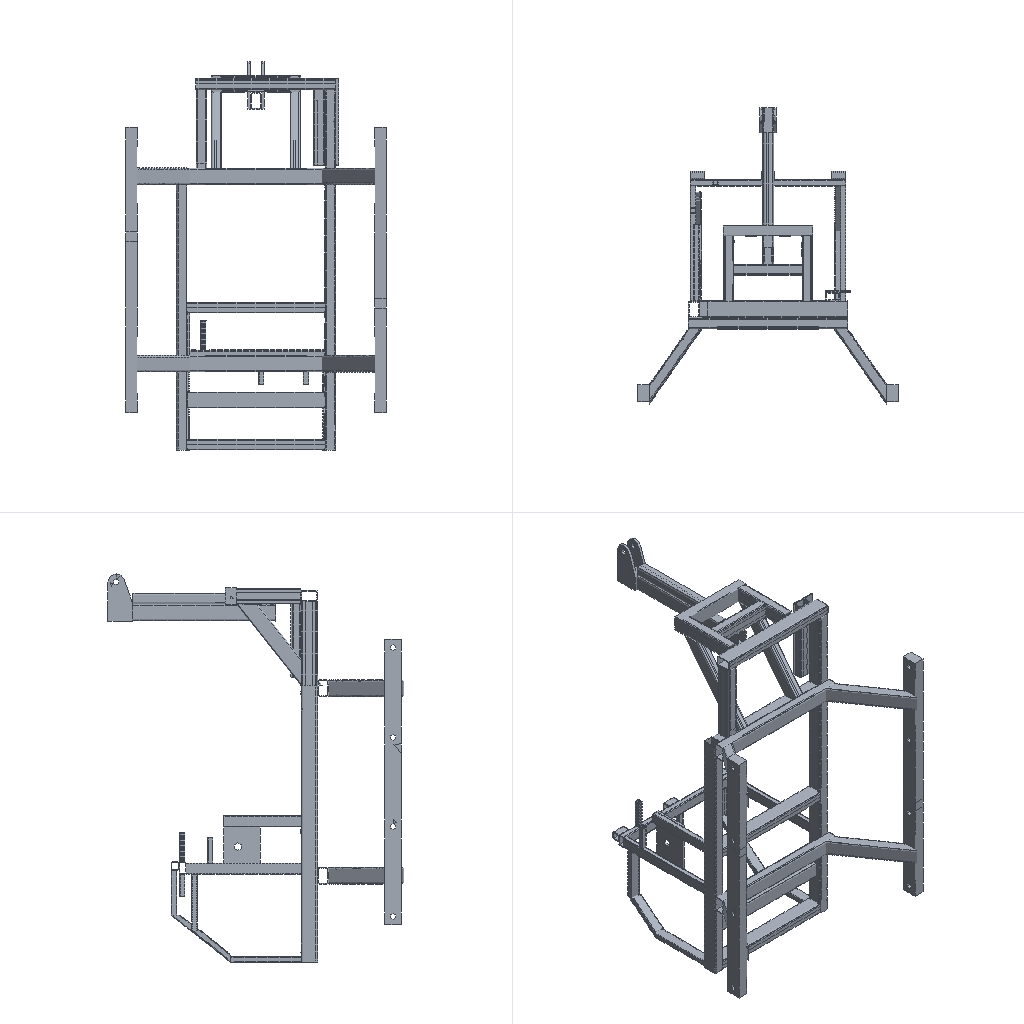Simulation study | ansys workbench
Set-up summary:
category,name,step,type,value,unit,region
solver,ansys_workbench
units,mm-N-s-tonne (MPa),,stated,"/units,MPA"
analysis,LS1,,modal,method=lanb; n_modes=12
load_step,LS1,LS1,modal
mesh,nodes,,,135459
mesh,elements,,,60243
element_type,SOLID187,,,42307
element_type,SOLID186,,,7352
element_type,TARGE170,,,5292
element_type,CONTA174,,,5292
material,Structural Steel,,E,200000,tonne s^-2 mm^-1
material,Structural Steel,,nu,0.3
material,Structural Steel,,density,7.85e-09,tonne mm^-3
material,Structural Steel,,conductivity,60.5,tonne mm s^-3 C^-1
material,Structural Steel,,specific_heat,4.34e+08,mm^2 s^-2 C^-1
material,Structural Steel,,cte,1.2e-05,C^-1
material,Structural Steel,,permeability,10000
material,Structural Steel,,resistivity,0.00017,ohm mm
bc,Fixed Supports,model,fixed,[dofs=ALL],,_FIXEDSU
contact,Contact Region,,bonded (always),element=CONTA174
contact,Contact Region 2,,bonded (always),element=CONTA174
contact,Contact Region 3,,bonded (always),element=CONTA174
contact,Contact Region 4,,bonded (always),element=CONTA174
contact,Contact Region 5,,bonded (always),element=CONTA174
contact,Contact Region 6,,bonded (always),element=CONTA174
contact,Contact Region 7,,bonded (always),element=CONTA174
contact,Contact Region 8,,bonded (always),element=CONTA174
contact,Contact Region 9,,bonded (always),element=CONTA174
contact,Contact Region 10,,bonded (always),element=CONTA174
contact,Contact Region 11,,bonded (always),element=CONTA174
contact,Contact Region 12,,bonded (always),element=CONTA174
contact,Contact Region 13,,bonded (always),element=CONTA174
contact,Contact Region 14,,bonded (always),element=CONTA174
contact,Contact Region 15,,bonded (always),element=CONTA174
contact,Contact Region 16,,bonded (always),element=CONTA174
contact,Contact Region 17,,bonded (always),element=CONTA174
contact,Contact Region 18,,bonded (always),element=CONTA174
contact,Contact Region 19,,bonded (always),element=CONTA174
contact,Contact Region 20,,bonded (always),element=CONTA174
contact,Contact Region 21,,bonded (always),element=CONTA174
contact,Contact Region 22,,bonded (always),element=CONTA174
contact,Contact Region 23,,bonded (always),element=CONTA174
contact,Contact Region 24,,bonded (always),element=CONTA174
contact,Contact Region 25,,bonded (always),element=CONTA174
contact,Contact Region 26,,bonded (always),element=CONTA174
contact,Contact Region 27,,bonded (always),element=CONTA174
contact,Contact Region 28,,bonded (always),element=CONTA174
contact,Contact Region 29,,bonded (always),element=CONTA174
contact,Contact Region 30,,bonded (always),element=CONTA174
contact,Contact Region 31,,bonded (always),element=CONTA174
contact,Contact Region 32,,bonded (always),element=CONTA174
contact,Contact Region 33,,bonded (always),element=CONTA174
contact,Contact Region 34,,bonded (always),element=CONTA174
contact,Contact Region 35,,bonded (always),element=CONTA174
contact,Contact Region 36,,bonded (always),element=CONTA174
contact,Contact Region 37,,bonded (always),element=CONTA174
contact,Contact Region 38,,bonded (always),element=CONTA174
contact,Contact Region 39,,bonded (always),element=CONTA174
contact,Contact Region 40,,bonded (always),element=CONTA174
contact,Contact Region 41,,bonded (always),element=CONTA174
contact,Contact Region 42,,bonded (always),element=CONTA174
contact,Contact Region 43,,bonded (always),element=CONTA174
contact,Contact Region 44,,bonded (always),element=CONTA174
contact,Contact Region 45,,bonded (always),element=CONTA174
contact,Contact Region 46,,bonded (always),element=CONTA174
contact,Contact Region 47,,bonded (always),element=CONTA174
contact,Contact Region 48,,bonded (always),element=CONTA174
contact,Contact Region 49,,bonded (always),element=CONTA174
contact,Contact Region 50,,bonded (always),element=CONTA174
contact,Contact Region 51,,bonded (always),element=CONTA174
contact,Contact Region 52,,bonded (always),element=CONTA174
contact,Contact Region 53,,bonded (always),element=CONTA174
contact,Contact Region 54,,bonded (always),element=CONTA174
contact,Contact Region 55,,bonded (always),element=CONTA174
contact,Contact Region 56,,bonded (always),element=CONTA174
contact,Contact Region 57,,bonded (always),element=CONTA174
contact,Contact Region 58,,bonded (always),element=CONTA174
contact,Contact Region 59,,bonded (always),element=CONTA174
contact,Contact Region 60,,bonded (always),element=CONTA174
contact,Contact Region 61,,bonded (always),element=CONTA174
contact,Contact Region 62,,bonded (always),element=CONTA174
contact,Contact Region 63,,bonded (always),element=CONTA174
contact,Contact Region 64,,bonded (always),element=CONTA174
contact,Contact Region 65,,bonded (always),element=CONTA174
contact,Contact Region 66,,bonded (always),element=CONTA174
contact,Contact Region 67,,bonded (always),element=CONTA174
named_set,_FIXEDSU,,node,216
Ansys APDL input file, long lists of numbers shortened:
/batch
/config,noeldb,1     ! force off writing results to database
*get,_wallstrt,active,,time,wall
! ANSYS input file written by Workbench version 2022 R1
! File used for geometry attach:
/title,wbnew--__ (B5)
! ****** Begin Custom Load Command Snippet ******
/COM, ACT Extensions:
/COM,     LSDYNA, 2021.1
/COM,
! ****** End   Custom Load Command Snippet ******
*DIM,_wb_ProjectScratch_dir,string,248
_wb_ProjectScratch_dir(1) = ''
*DIM,_wb_SolverFiles_dir,string,248
_wb_SolverFiles_dir(1) = ''
*DIM,_wb_userfiles_dir,string,248
_wb_userfiles_dir(1) = ''
/com,--- Data in consistent NMM units. See Solving Units in the help system for more information.
/units,MPA
/nopr
/wb,file,start              !  signify a WB generated input file
/prep7
! Turn off shape checking because checks already performed inside WB mesher.
! See help system for more information.
SHPP,OFF,,NOWARN
/nolist
etcon,set             ! allow ANSYS to choose best KEYOP's for 180x elements, resets any applicable keyopt to MAPDL defaults
/com,*********** Nodes for the whole assembly ***********
nblock,3,,149004
(1i9,3e20.9e3)
        1    -5.127313953E+02     3.050000000E+02    -7.650000000E+02
! (135458 more lines like these left out)
-1
/wb,elem,start            !  set before creation of elements
/com,*********** Elements for Body 1 "1290___<___>|______ 60 X 40 X 3.2(1)" ***********
et,1,187
eblock,19,solid,,5298
(19i9)
        1        1        1        1        0        0        0        0       10        0    25062    85257    86308    85943    85275    87073    92272    87072    87068
! (10595 more lines like these left out)
-1
/com,*********** Elements for Body 2 "500___<___>|______ 60 X 40 X 3.2(1)" ***********
et,2,186
keyo,2,2,1          ! set full integration on SOLID186
eblock,19,solid,,330
(19i9)
        2        2        2        2        0        0        0        0       20        0    17793    58415    58420    58683    58418    58480    58475    58684    58477
! (659 more lines like these left out)
-1
/com,*********** Elements for Body 3 "490___<___>|______ 60 X 40 X 3.2(1)" ***********
et,3,186
keyo,3,2,1          ! set full integration on SOLID186
eblock,19,solid,,300
(19i9)
        3        3        3        3        0        0        0        0       20        0    18123    60525    60530    60773    60528    60584    60579    60774    60581
! (599 more lines like these left out)
-1
/com,*********** Elements for Body 4 "990___<___>|______ 60 X 40 X 3.2(1)" ***********
et,4,187
eblock,19,solid,,4671
(19i9)
        4        4        4        4        0        0        0        0       10        0    41556   119381   119483   119740   120479   123434   124373   123436   123439
! (9341 more lines like these left out)
-1
/com,*********** Elements for Body 5 "490___<___>|______ 60 X 40 X 3.2(1)[2]" ***********
et,5,186
keyo,5,2,1          ! set full integration on SOLID186
eblock,19,solid,,300
(19i9)
        5        5        5        5        0        0        0        0       20        0     6107    26432    26437    26680    26435    26491    26486    26681    26488
! (599 more lines like these left out)
-1
! (41 more sections like these left out)
/wb,elem,end               !  done creating elements
/com,*********** Send User Defined Coordinate System(s) ***********
csys,0
toffst,273.15,  ! Temperature offset from absolute zero
/com,*********** Set Reference Temperature ***********
tref,22.
/wb,mat,start              !  starting to send materials
/com,*********** Send Materials ***********
Temperature = 'TEMP' ! Temperature
MP,DENS,1,7.85e-09,	! tonne mm^-3
MP,ALPX,1,1.2e-05,	! C^-1
MP,C,1,434000000,	! mm^2 s^-2 C^-1
MP,KXX,1,60.5,	! tonne mm s^-3 C^-1
MP,RSVX,1,0.00017,	! ohm mm
MP,EX,1,200000,	! tonne s^-2 mm^-1
MP,NUXY,1,0.3,
MP,MURX,1,10000,
Temperature = 'TEMP' ! Temperature
MP,DENS,2,7.85e-09,	! tonne mm^-3
MP,ALPX,2,1.2e-05,	! C^-1
MP,C,2,434000000,	! mm^2 s^-2 C^-1
MP,KXX,2,60.5,	! tonne mm s^-3 C^-1
MP,RSVX,2,0.00017,	! ohm mm
MP,EX,2,200000,	! tonne s^-2 mm^-1
MP,NUXY,2,0.3,
MP,MURX,2,10000,
Temperature = 'TEMP' ! Temperature
MP,DENS,3,7.85e-09,	! tonne mm^-3
MP,ALPX,3,1.2e-05,	! C^-1
MP,C,3,434000000,	! mm^2 s^-2 C^-1
MP,KXX,3,60.5,	! tonne mm s^-3 C^-1
MP,RSVX,3,0.00017,	! ohm mm
MP,EX,3,200000,	! tonne s^-2 mm^-1
MP,NUXY,3,0.3,
MP,MURX,3,10000,
Temperature = 'TEMP' ! Temperature
MP,DENS,4,7.85e-09,	! tonne mm^-3
MP,ALPX,4,1.2e-05,	! C^-1
MP,C,4,434000000,	! mm^2 s^-2 C^-1
MP,KXX,4,60.5,	! tonne mm s^-3 C^-1
MP,RSVX,4,0.00017,	! ohm mm
MP,EX,4,200000,	! tonne s^-2 mm^-1
MP,NUXY,4,0.3,
MP,MURX,4,10000,
Temperature = 'TEMP' ! Temperature
MP,DENS,5,7.85e-09,	! tonne mm^-3
MP,ALPX,5,1.2e-05,	! C^-1
MP,C,5,434000000,	! mm^2 s^-2 C^-1
MP,KXX,5,60.5,	! tonne mm s^-3 C^-1
MP,RSVX,5,0.00017,	! ohm mm
MP,EX,5,200000,	! tonne s^-2 mm^-1
MP,NUXY,5,0.3,
MP,MURX,5,10000,
Temperature = 'TEMP' ! Temperature
MP,DENS,6,7.85e-09,	! tonne mm^-3
MP,ALPX,6,1.2e-05,	! C^-1
MP,C,6,434000000,	! mm^2 s^-2 C^-1
MP,KXX,6,60.5,	! tonne mm s^-3 C^-1
MP,RSVX,6,0.00017,	! ohm mm
MP,EX,6,200000,	! tonne s^-2 mm^-1
MP,NUXY,6,0.3,
MP,MURX,6,10000,
Temperature = 'TEMP' ! Temperature
MP,DENS,7,7.85e-09,	! tonne mm^-3
MP,ALPX,7,1.2e-05,	! C^-1
MP,C,7,434000000,	! mm^2 s^-2 C^-1
MP,KXX,7,60.5,	! tonne mm s^-3 C^-1
MP,RSVX,7,0.00017,	! ohm mm
MP,EX,7,200000,	! tonne s^-2 mm^-1
MP,NUXY,7,0.3,
MP,MURX,7,10000,
Temperature = 'TEMP' ! Temperature
MP,DENS,8,7.85e-09,	! tonne mm^-3
MP,ALPX,8,1.2e-05,	! C^-1
MP,C,8,434000000,	! mm^2 s^-2 C^-1
MP,KXX,8,60.5,	! tonne mm s^-3 C^-1
MP,RSVX,8,0.00017,	! ohm mm
MP,EX,8,200000,	! tonne s^-2 mm^-1
MP,NUXY,8,0.3,
MP,MURX,8,10000,
Temperature = 'TEMP' ! Temperature
MP,DENS,9,7.85e-09,	! tonne mm^-3
MP,ALPX,9,1.2e-05,	! C^-1
MP,C,9,434000000,	! mm^2 s^-2 C^-1
MP,KXX,9,60.5,	! tonne mm s^-3 C^-1
MP,RSVX,9,0.00017,	! ohm mm
MP,EX,9,200000,	! tonne s^-2 mm^-1
! (335 more lines like these left out)
/wb,mat,end                !  done sending materials
!************************* Model Summary ********************
!1290___<___>|______ 60 X 40 X 3.2(1),	结构钢,	matid,	1
!500___<___>|______ 60 X 40 X 3.2(1),	结构钢,	matid,	2
!490___<___>|______ 60 X 40 X 3.2(1),	结构钢,	matid,	3
! (45 more lines like these left out)
*get,_xmin,node,,mnloc,x
*get,_ymin,node,,mnloc,y
*get,_zmin,node,,mnloc,z
*get,_xmax,node,,mxloc,x
*get,_ymax,node,,mxloc,y
*get,_zmax,node,,mxloc,z
_ASMDIAG=(_xmax-_xmin)*(_xmax-_xmin)+(_ymax-_ymin)*(_ymax-_ymin)+(_zmax-_zmin)*(_zmax-_zmin)
_ASMDIAG=SQRT(_ASMDIAG)
/wb,contact,start          !  starting to send contact
/com,*********** Create Contact "接触区域" ***********
/com,            Real Constant Set For Above Contact Is 48 & 47
*set,tid,48
*set,cid,47
r,tid
r,cid
et,tid,170
et,cid,174
eblock,10,,,64
(15i9)
    92008       48       48       48        0    85579    85566    85925    85925    89467    89470    85925    89529
! (63 more lines like these left out)
-1
eblock,10,,,64
(15i9)
    92072       47       47       47        0    85579    85566    85925    85925    89467    89470    85925    89529
! (63 more lines like these left out)
-1
eblock,10,,,16
(15i9)
    92136       47       48       47        0    58607    58595    58594    58606    59591    59587    59588    59622
! (15 more lines like these left out)
-1
eblock,10,,,16
(15i9)
    92152       48       47       48        0    58607    58595    58594    58606    59591    59587    59588    59622
! (15 more lines like these left out)
-1
keyo,cid,8,2               ! auto create asymmetric contact (from Program Controlled setting)
keyo,cid,10,0              ! adjust contact stiffness each NR iteration (from Program Controlled setting)
keyo,cid,12,5              ! bonded always
keyo,cid,18,1              ! small sliding turned on by application
keyo,cid,2,0               ! augmented Lagrange (from Program Controlled setting)
keyo,cid,4,0               ! on Gauss point (from Program Controlled setting)
keyo,cid,9,1               ! ignore initial gaps/penetration
keyo,cid,7,0               ! No Prediction
rmod,tid,3,10.      ! FKN
rmod,tid,5,0.       ! ICONT
rmod,tid,6,0.       ! PINB
rmod,tid,10,0.      ! CNOF
rmod,tid,12,0.      ! FKT
rmod,tid,36,161     ! WB DSID
rmod,cid,3,10.      ! FKN
rmod,cid,5,0.       ! ICONT
rmod,cid,6,0.       ! PINB
rmod,cid,10,0.      ! CNOF
rmod,cid,12,0.      ! FKT
rmod,cid,36,161     ! WB DSID
/com,*********** Create Contact "接触区域 2" ***********
/com,            Real Constant Set For Above Contact Is 50 & 49
*set,tid,50
*set,cid,49
r,tid
r,cid
et,tid,170
et,cid,174
eblock,10,,,53
(15i9)
    92168       50       50       50        0    85654    85635    86052    86052    89917    89923    86052    90118
! (52 more lines like these left out)
-1
eblock,10,,,53
(15i9)
    92221       49       49       49        0    85654    85635    86052    86052    89917    89923    86052    90118
! (52 more lines like these left out)
-1
eblock,10,,,30
(15i9)
    92274       49       50       49        0    60674    60582    60646    60646    61300    61299    60646    61472
! (29 more lines like these left out)
-1
eblock,10,,,30
(15i9)
    92304       50       49       50        0    60674    60582    60646    60646    61300    61299    60646    61472
! (29 more lines like these left out)
-1
keyo,cid,8,2               ! auto create asymmetric contact (from Program Controlled setting)
keyo,cid,10,0              ! adjust contact stiffness each NR iteration (from Program Controlled setting)
keyo,cid,12,5              ! bonded always
keyo,cid,18,1              ! small sliding turned on by application
keyo,cid,2,0               ! augmented Lagrange (from Program Controlled setting)
keyo,cid,4,0               ! on Gauss point (from Program Controlled setting)
keyo,cid,9,1               ! ignore initial gaps/penetration
keyo,cid,7,0               ! No Prediction
rmod,tid,3,10.      ! FKN
rmod,tid,5,0.       ! ICONT
rmod,tid,6,0.       ! PINB
rmod,tid,10,0.      ! CNOF
rmod,tid,12,0.      ! FKT
rmod,tid,36,164     ! WB DSID
rmod,cid,3,10.      ! FKN
rmod,cid,5,0.       ! ICONT
rmod,cid,6,0.       ! PINB
rmod,cid,10,0.      ! CNOF
rmod,cid,12,0.      ! FKT
rmod,cid,36,164     ! WB DSID
/com,*********** Create Contact "接触区域 3" ***********
/com,            Real Constant Set For Above Contact Is 52 & 51
*set,tid,52
*set,cid,51
r,tid
r,cid
et,tid,170
et,cid,174
eblock,10,,,36
(15i9)
    92334       52       52       52        0    86039    85647    86075    86075    90045    90047    86075    92858
! (35 more lines like these left out)
-1
eblock,10,,,36
(15i9)
    92370       51       51       51        0    86039    85647    86075    86075    90045    90047    86075    92858
! (35 more lines like these left out)
-1
eblock,10,,,30
(15i9)
    92406       51       52       51        0    26581    26489    26553    26553    27207    27206    26553    27379
! (29 more lines like these left out)
-1
eblock,10,,,30
(15i9)
    92436       52       51       52        0    26581    26489    26553    26553    27207    27206    26553    27379
! (29 more lines like these left out)
-1
keyo,cid,8,2               ! auto create asymmetric contact (from Program Controlled setting)
keyo,cid,10,0              ! adjust contact stiffness each NR iteration (from Program Controlled setting)
keyo,cid,12,5              ! bonded always
keyo,cid,18,1              ! small sliding turned on by application
keyo,cid,2,0               ! augmented Lagrange (from Program Controlled setting)
keyo,cid,4,0               ! on Gauss point (from Program Controlled setting)
keyo,cid,9,1               ! ignore initial gaps/penetration
keyo,cid,7,0               ! No Prediction
rmod,tid,3,10.      ! FKN
rmod,tid,5,0.       ! ICONT
rmod,tid,6,0.       ! PINB
rmod,tid,10,0.      ! CNOF
rmod,tid,12,0.      ! FKT
rmod,tid,36,167     ! WB DSID
rmod,cid,3,10.      ! FKN
rmod,cid,5,0.       ! ICONT
rmod,cid,6,0.       ! PINB
rmod,cid,10,0.      ! CNOF
rmod,cid,12,0.      ! FKT
rmod,cid,36,167     ! WB DSID
/com,*********** Create Contact "接触区域 4" ***********
/com,            Real Constant Set For Above Contact Is 54 & 53
*set,tid,54
*set,cid,53
r,tid
r,cid
et,tid,170
et,cid,174
eblock,10,,,37
(15i9)
    92466       54       54       54        0    86027    85641    86063    86063    89983    89985    86063    92810
! (36 more lines like these left out)
-1
eblock,10,,,37
(15i9)
    92503       53       53       53        0    86027    85641    86063    86063    89983    89985    86063    92810
! (36 more lines like these left out)
-1
eblock,10,,,30
(15i9)
    92540       53       54       53        0    51040    50948    51012    51012    51666    51665    51012    51838
! (29 more lines like these left out)
-1
eblock,10,,,30
(15i9)
    92570       54       53       54        0    51040    50948    51012    51012    51666    51665    51012    51838
! (29 more lines like these left out)
-1
keyo,cid,8,2               ! auto create asymmetric contact (from Program Controlled setting)
keyo,cid,10,0              ! adjust contact stiffness each NR iteration (from Program Controlled setting)
keyo,cid,12,5              ! bonded always
keyo,cid,18,1              ! small sliding turned on by application
keyo,cid,2,0               ! augmented Lagrange (from Program Controlled setting)
keyo,cid,4,0               ! on Gauss point (from Program Controlled setting)
keyo,cid,9,1               ! ignore initial gaps/penetration
keyo,cid,7,0               ! No Prediction
rmod,tid,3,10.      ! FKN
rmod,tid,5,0.       ! ICONT
rmod,tid,6,0.       ! PINB
rmod,tid,10,0.      ! CNOF
rmod,tid,12,0.      ! FKT
rmod,tid,36,170     ! WB DSID
rmod,cid,3,10.      ! FKN
rmod,cid,5,0.       ! ICONT
rmod,cid,6,0.       ! PINB
rmod,cid,10,0.      ! CNOF
rmod,cid,12,0.      ! FKT
rmod,cid,36,170     ! WB DSID
/com,*********** Create Contact "接触区域 5" ***********
/com,            Real Constant Set For Above Contact Is 56 & 55
*set,tid,56
*set,cid,55
r,tid
r,cid
et,tid,170
et,cid,174
eblock,10,,,36
(15i9)
    92600       56       56       56        0    85261    85950    86756    86756    87104    92316    86756    87107
! (35 more lines like these left out)
-1
eblock,10,,,36
(15i9)
    92636       55       55       55        0    85261    85950    86756    86756    87104    92316    86756    87107
! (35 more lines like these left out)
-1
eblock,10,,,8
(15i9)
    92672       55       56       55        0    62557    62558    62568    62591    63370    63372    63411    63371
! (7 more lines like these left out)
-1
eblock,10,,,8
(15i9)
    92680       56       55       56        0    62557    62558    62568    62591    63370    63372    63411    63371
! (7 more lines like these left out)
-1
keyo,cid,8,2               ! auto create asymmetric contact (from Program Controlled setting)
keyo,cid,10,0              ! adjust contact stiffness each NR iteration (from Program Controlled setting)
keyo,cid,12,5              ! bonded always
keyo,cid,18,1              ! small sliding turned on by application
keyo,cid,2,0               ! augmented Lagrange (from Program Controlled setting)
keyo,cid,4,0               ! on Gauss point (from Program Controlled setting)
keyo,cid,9,1               ! ignore initial gaps/penetration
keyo,cid,7,0               ! No Prediction
rmod,tid,3,10.      ! FKN
rmod,tid,5,0.       ! ICONT
rmod,tid,6,0.       ! PINB
rmod,tid,10,0.      ! CNOF
rmod,tid,12,0.      ! FKT
rmod,tid,36,173     ! WB DSID
rmod,cid,3,10.      ! FKN
rmod,cid,5,0.       ! ICONT
rmod,cid,6,0.       ! PINB
rmod,cid,10,0.      ! CNOF
rmod,cid,12,0.      ! FKT
rmod,cid,36,173     ! WB DSID
! (62 more sections like these left out)
/wb,contact,end            !  done creating contacts
/golist
/wb,load,start             !  starting to send loads
/com,*********** Fixed Supports ***********
CMBLOCK,_FIXEDSU,NODE,      216
(8i10)
     72560     72561     72562     72563     72564     72565     72566     72567
! (26 more lines like these left out)
cmsel,s,_FIXEDSU
d,all,all
nsel,all
/gst,on,on
fini
*get,_numnode,node,0,count
*get,_numelem,elem,0,count
*get, _MAXELEMNUM, elem, 0, NUM, MAX
*get, _MAXNODENUM, node, 0, NUM, MAX
*get, _MAXELEMTYPE, etyp, 0, NUM, MAX
*get, _MAXREALCONST, real, 0, NUM, MAX
/go
/wb,load,end               !  done creating loads
/com,--- Number of total nodes = %_numnode%
/com,--- Number of contact elements = 10584
/com,--- Number of spring elements = 0
/com,--- Number of bearing elements = 0
/com,--- Number of solid elements = 49659
/com,--- Number of condensed parts = 0
/com,--- Number of total elements = %_numelem%
*get,_wallbsol,active,,time,wall
/solu
antype,2                   ! modal analysis
_thickRatio=0.37    ! Ratio of thick parts in the model
modopt,lanb,12
outres,erase
outres,all,none
outres,nsol,all
outres,etmp,all
mxpand                    ! default expand in case of complex solution
dmpopt,esav,no
dmpopt,emat,no
dmpopt,full,no
! *********** WB SOLVE COMMAND ***********
! check interactive state
*get,ANSINTER_,active,,int
*if,ANSINTER_,ne,0,then
/eof
*endif
solve
/com *************** Write FE CONNECTORS *********
CEWRITE,file,ce,,INTE
*get,_nmodalsolproc,active,0,numcpu
fini
/nopr
*get,_numnode,node,0,count
*get,_numelem,elem,0,count
*get, _MAXELEMNUM, elem, 0, NUM, MAX
*get, _MAXNODENUM, node, 0, NUM, MAX,,,INTERNAL
*get, _MAXELEMTYPE, etyp, 0, NUM, MAX
*get, _MAXREALCONST, real, 0, NUM, MAX
/gopr
*get,_wallasol,active,,time,wall
/post1
/nopr
*dim,_direction,CHAR,6,1
_direction(1) = 'X'
_direction(2) = 'Y'
_direction(3) = 'Z'
_direction(4) = 'ROTX'
_direction(5) = 'ROTY'
_direction(6) = 'ROTZ'
*get,_lastLS,active,0,set,LSTP
*get,_beginset,active,0,set,nset,first,_lastLS
*get,_endset,active,0,set,nset,last,_lastLS
_nummodes = 0
*if,_endset,gt,0,then
_nummodes = _endset - _beginset + 1
*endif
*do,i_mode,1,_nummodes
   *do,j_component,1,6
			*get,PFACT_%i_mode%_%j_component%,MODE,%i_mode%,PFACT,,DIREC,_direction(%j_component%)
   *enddo
*enddo
*dim,_tmdirection,CHAR,6,1
_tmdirection(1) = 'X'
_tmdirection(2) = 'Y'
_tmdirection(3) = 'Z'
_tmdirection(4) = 'X'
_tmdirection(5) = 'Y'
_tmdirection(6) = 'Z'
*do,j_component,1,6
    *if,j_component,gt,3,then
        *get,TOTALMASS_%j_component%,ELEM,0,IOR,_tmdirection(%j_component%)
    *else
        *get,TOTALMASS_%j_component%,ELEM,0,MTOT,_tmdirection(%j_component%)
    *endif
*enddo
/gopr
xmlo,ENCODING,ISO-8859-1
xmlo,parm
/xml,parm,xml
fini
/gopr
*get,_walldone,active,,time,wall
_preptime=(_wallbsol-_wallstrt)*3600
_solvtime=(_wallasol-_wallbsol)*3600
_posttime=(_walldone-_wallasol)*3600
_totaltim=(_walldone-_wallstrt)*3600
*get,_dlbratio,active,0,solu,dlbr
*get,_combtime,active,0,solu,comb
*get,_ssmode,active,0,solu,ssmm
*get,_ndofs,active,0,solu,ndof
/fclean				!clean distributed files
/com,--- Total number of nodes = %_numnode%
/com,--- Total number of elements = %_numelem%
/com,--- Element load balance ratio = %_dlbratio%
/com,--- Time to combine distributed files = %_combtime%
/com,--- Sparse memory mode = %_ssmode%
/com,--- Number of DOF = %_ndofs%
/wb,file,end               ! done with WB generated input
Results summary:
result,analyses[0].index,,,1
result,analyses[0].system,,,SYS
result,analyses[0].deck,,,deck.dat
result,analyses[0].solve_status,,,completed
result,analyses[0].analysis_type,,,modal
result,analyses[0].physics,,,mechanical
result,analyses[0].unit_system,,,"NMM: mm, ton, N, s, mV, mA, degC"
result,analyses[0].n_sets,,,12
result,analyses[0].modal_frequencies_hz[1],,,56.265
result,analyses[0].modal_frequencies_hz[2],,,73.846
result,analyses[0].modal_frequencies_hz[3],,,80.156
result,analyses[0].modal_frequencies_hz[4],,,82.068
result,analyses[0].modal_frequencies_hz[5],,,83.608
result,analyses[0].modal_frequencies_hz[6],,,120.313
result,analyses[0].modal_frequencies_hz[7],,,130.69
result,analyses[0].modal_frequencies_hz[8],,,143.473
result,analyses[0].modal_frequencies_hz[9],,,148.303
result,analyses[0].modal_frequencies_hz[10],,,175.315
result,analyses[0].modal_frequencies_hz[11],,,188.429
result,analyses[0].modal_frequencies_hz[12],,,202.044